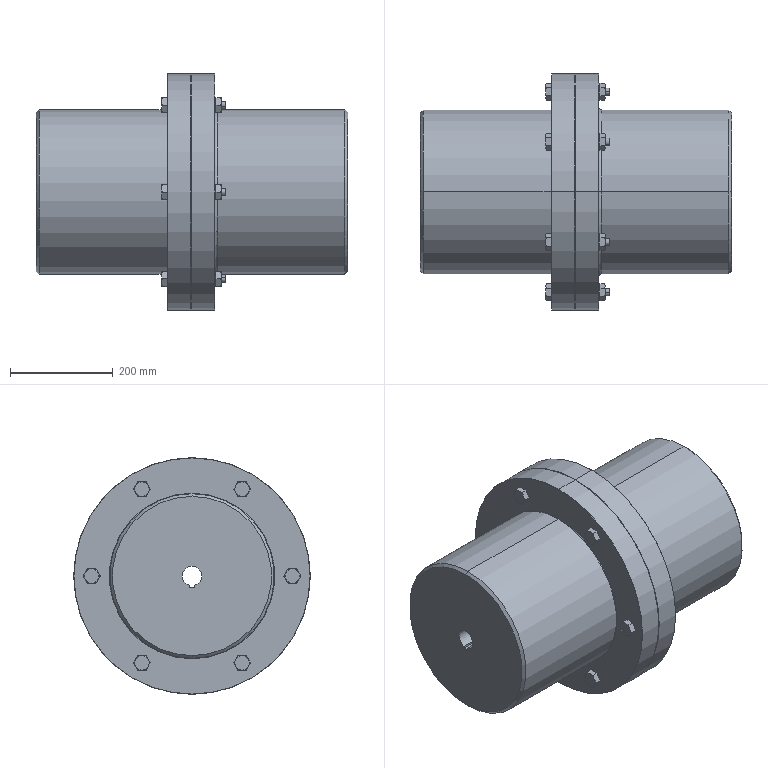Part | SolidWorks | features ICE 15, Chamfer 6, Revolution 3, CirPattern 2, Fillet 2 | 1 solid | 433 faces | box 605 x 460 x 460 mm | volume 55419022 mm3 | plane 223 | cone 144 | cylinder 62 | torus 4 | commonest cylinder face diameters 14 x36 28 x12 320 x7 460 x4 38 x3